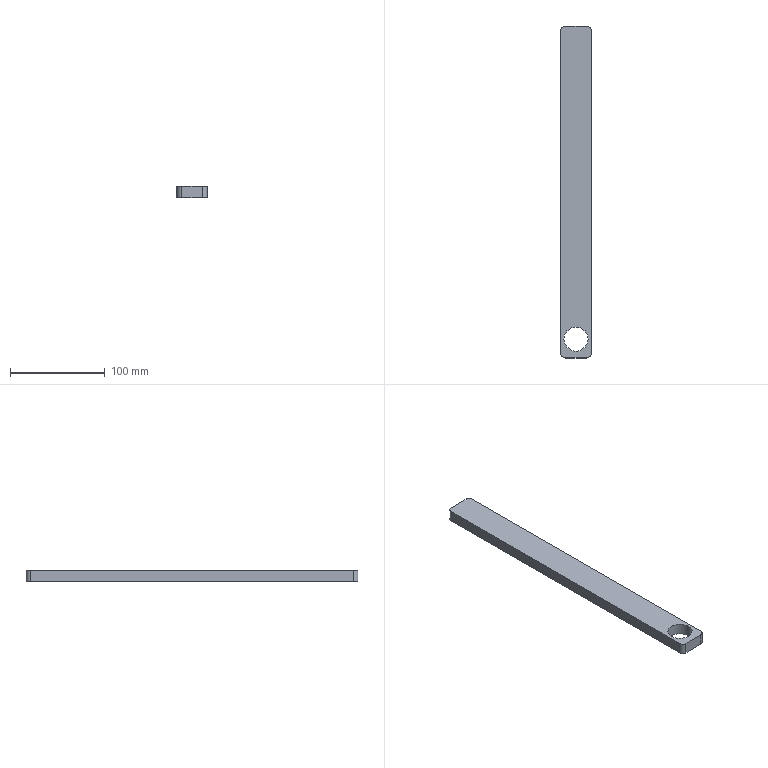Part | SolidWorks | features Extrusion 1 | 1 solid | 12 faces | box 32 x 350 x 12 mm | volume 128014 mm3 | cylinder 6 | plane 6 | commonest cylinder face diameters 10 x4 25.5 x2
STEP:
#1=CARTESIAN_POINT('',(3.25,20.,12.));
#2=VERTEX_POINT('',#1);
#3=CARTESIAN_POINT('',(28.75,20.,12.));
#4=VERTEX_POINT('',#3);
#5=CARTESIAN_POINT('',(16.,20.,12.));
#6=DIRECTION('',(0.,0.,1.));
#7=DIRECTION('',(1.,0.,0.));
#8=AXIS2_PLACEMENT_3D('',#5,#6,#7);
#9=CIRCLE('',#8,12.75);
#10=EDGE_CURVE('',#2,#4,#9,.T.);
#11=ORIENTED_EDGE('',*,*,#10,.T.);
#12=CARTESIAN_POINT('',(28.75,20.,0.));
#13=VERTEX_POINT('',#12);
#14=CARTESIAN_POINT('',(28.75,20.,12.));
#15=DIRECTION('',(0.,0.,-1.));
#16=VECTOR('',#15,1000.);
#17=LINE('',#14,#16);
#18=EDGE_CURVE('',#4,#13,#17,.T.);
#19=ORIENTED_EDGE('',*,*,#18,.T.);
#20=CARTESIAN_POINT('',(3.25,20.,0.));
#21=VERTEX_POINT('',#20);
#22=CARTESIAN_POINT('',(16.,20.,0.));
#23=DIRECTION('',(0.,0.,1.));
#24=DIRECTION('',(1.,0.,0.));
#25=AXIS2_PLACEMENT_3D('',#22,#23,#24);
#26=CIRCLE('',#25,12.75);
#27=EDGE_CURVE('',#21,#13,#26,.T.);
#28=ORIENTED_EDGE('',*,*,#27,.F.);
#29=CARTESIAN_POINT('',(3.25,20.,12.));
#30=DIRECTION('',(0.,0.,-1.));
#31=VECTOR('',#30,1000.);
#32=LINE('',#29,#31);
#33=EDGE_CURVE('',#2,#21,#32,.T.);
#34=ORIENTED_EDGE('',*,*,#33,.F.);
#35=EDGE_LOOP('',(#11,#19,#28,#34));
#36=FACE_OUTER_BOUND('',#35,.T.);
#37=CARTESIAN_POINT('',(16.,20.,12.));
#38=DIRECTION('',(0.,0.,-1.));
#39=DIRECTION('',(-1.,0.,0.));
#40=AXIS2_PLACEMENT_3D('',#37,#38,#39);
#41=CYLINDRICAL_SURFACE('',#40,12.75);
#42=ADVANCED_FACE('',(#36),#41,.F.);
#43=CARTESIAN_POINT('',(27.,0.,12.));
#44=VERTEX_POINT('',#43);
#45=CARTESIAN_POINT('',(32.,5.,12.));
#46=VERTEX_POINT('',#45);
#47=CARTESIAN_POINT('',(27.,5.,12.));
#48=DIRECTION('',(0.,0.,1.));
#49=DIRECTION('',(1.,0.,0.));
#50=AXIS2_PLACEMENT_3D('',#47,#48,#49);
#51=CIRCLE('',#50,5.);
#52=EDGE_CURVE('',#44,#46,#51,.T.);
#53=ORIENTED_EDGE('',*,*,#52,.T.);
#54=CARTESIAN_POINT('',(32.,345.,12.));
#55=VERTEX_POINT('',#54);
#56=CARTESIAN_POINT('',(32.,5.,12.));
#57=DIRECTION('',(0.,1.,0.));
#58=VECTOR('',#57,1000.);
#59=LINE('',#56,#58);
#60=EDGE_CURVE('',#46,#55,#59,.T.);
#61=ORIENTED_EDGE('',*,*,#60,.T.);
#62=CARTESIAN_POINT('',(27.,350.,12.));
#63=VERTEX_POINT('',#62);
#64=CARTESIAN_POINT('',(27.,345.,12.));
#65=DIRECTION('',(0.,0.,1.));
#66=DIRECTION('',(-1.,0.,0.));
#67=AXIS2_PLACEMENT_3D('',#64,#65,#66);
#68=CIRCLE('',#67,5.);
#69=EDGE_CURVE('',#55,#63,#68,.T.);
#70=ORIENTED_EDGE('',*,*,#69,.T.);
#71=CARTESIAN_POINT('',(5.,350.,12.));
#72=VERTEX_POINT('',#71);
#73=CARTESIAN_POINT('',(5.,350.,12.));
#74=DIRECTION('',(-1.,0.,0.));
#75=VECTOR('',#74,1000.);
#76=LINE('',#73,#75);
#77=EDGE_CURVE('',#63,#72,#76,.T.);
#78=ORIENTED_EDGE('',*,*,#77,.T.);
#79=CARTESIAN_POINT('',(0.,345.,12.));
#80=VERTEX_POINT('',#79);
#81=CARTESIAN_POINT('',(5.,345.,12.));
#82=DIRECTION('',(0.,0.,1.));
#83=DIRECTION('',(-1.,0.,0.));
#84=AXIS2_PLACEMENT_3D('',#81,#82,#83);
#85=CIRCLE('',#84,5.);
#86=EDGE_CURVE('',#72,#80,#85,.T.);
#87=ORIENTED_EDGE('',*,*,#86,.T.);
#88=CARTESIAN_POINT('',(0.,5.,12.));
#89=VERTEX_POINT('',#88);
#90=CARTESIAN_POINT('',(0.,5.,12.));
#91=DIRECTION('',(0.,-1.,0.));
#92=VECTOR('',#91,1000.);
#93=LINE('',#90,#92);
#94=EDGE_CURVE('',#80,#89,#93,.T.);
#95=ORIENTED_EDGE('',*,*,#94,.T.);
#96=CARTESIAN_POINT('',(5.,0.,12.));
#97=VERTEX_POINT('',#96);
#98=CARTESIAN_POINT('',(5.,5.,12.));
#99=DIRECTION('',(0.,0.,1.));
#100=DIRECTION('',(-1.,0.,0.));
#101=AXIS2_PLACEMENT_3D('',#98,#99,#100);
#102=CIRCLE('',#101,5.);
#103=EDGE_CURVE('',#89,#97,#102,.T.);
#104=ORIENTED_EDGE('',*,*,#103,.T.);
#105=CARTESIAN_POINT('',(5.,0.,12.));
#106=DIRECTION('',(1.,0.,0.));
#107=VECTOR('',#106,1000.);
#108=LINE('',#105,#107);
#109=EDGE_CURVE('',#97,#44,#108,.T.);
#110=ORIENTED_EDGE('',*,*,#109,.T.);
#111=EDGE_LOOP('',(#53,#61,#70,#78,#87,#95,#104,#110));
#112=FACE_OUTER_BOUND('',#111,.T.);
#113=ORIENTED_EDGE('',*,*,#10,.F.);
#114=CARTESIAN_POINT('',(16.,20.,12.));
#115=DIRECTION('',(0.,0.,1.));
#116=DIRECTION('',(1.,0.,0.));
#117=AXIS2_PLACEMENT_3D('',#114,#115,#116);
#118=CIRCLE('',#117,12.75);
#119=EDGE_CURVE('',#4,#2,#118,.T.);
#120=ORIENTED_EDGE('',*,*,#119,.F.);
#121=EDGE_LOOP('',(#113,#120));
#122=FACE_BOUND('',#121,.T.);
#123=CARTESIAN_POINT('',(27.,5.,12.));
#124=DIRECTION('',(0.,0.,1.));
#125=DIRECTION('',(1.,0.,0.));
#126=AXIS2_PLACEMENT_3D('',#123,#124,#125);
#127=PLANE('',#126);
#128=ADVANCED_FACE('',(#112,#122),#127,.T.);
#129=CARTESIAN_POINT('',(27.,0.,0.));
#130=VERTEX_POINT('',#129);
#131=CARTESIAN_POINT('',(32.,5.,0.));
#132=VERTEX_POINT('',#131);
#133=CARTESIAN_POINT('',(27.,5.,0.));
#134=DIRECTION('',(0.,0.,1.));
#135=DIRECTION('',(1.,0.,0.));
#136=AXIS2_PLACEMENT_3D('',#133,#134,#135);
#137=CIRCLE('',#136,5.);
#138=EDGE_CURVE('',#130,#132,#137,.T.);
#139=ORIENTED_EDGE('',*,*,#138,.F.);
#140=CARTESIAN_POINT('',(5.,0.,0.));
#141=VERTEX_POINT('',#140);
#142=CARTESIAN_POINT('',(5.,0.,0.));
#143=DIRECTION('',(1.,0.,0.));
#144=VECTOR('',#143,1000.);
#145=LINE('',#142,#144);
#146=EDGE_CURVE('',#141,#130,#145,.T.);
#147=ORIENTED_EDGE('',*,*,#146,.F.);
#148=CARTESIAN_POINT('',(0.,5.,0.));
#149=VERTEX_POINT('',#148);
#150=CARTESIAN_POINT('',(5.,5.,0.));
#151=DIRECTION('',(0.,0.,1.));
#152=DIRECTION('',(-1.,0.,0.));
#153=AXIS2_PLACEMENT_3D('',#150,#151,#152);
#154=CIRCLE('',#153,5.);
#155=EDGE_CURVE('',#149,#141,#154,.T.);
#156=ORIENTED_EDGE('',*,*,#155,.F.);
#157=CARTESIAN_POINT('',(0.,345.,0.));
#158=VERTEX_POINT('',#157);
#159=CARTESIAN_POINT('',(0.,5.,0.));
#160=DIRECTION('',(0.,-1.,0.));
#161=VECTOR('',#160,1000.);
#162=LINE('',#159,#161);
#163=EDGE_CURVE('',#158,#149,#162,.T.);
#164=ORIENTED_EDGE('',*,*,#163,.F.);
#165=CARTESIAN_POINT('',(5.,350.,0.));
#166=VERTEX_POINT('',#165);
#167=CARTESIAN_POINT('',(5.,345.,0.));
#168=DIRECTION('',(0.,0.,1.));
#169=DIRECTION('',(-1.,0.,0.));
#170=AXIS2_PLACEMENT_3D('',#167,#168,#169);
#171=CIRCLE('',#170,5.);
#172=EDGE_CURVE('',#166,#158,#171,.T.);
#173=ORIENTED_EDGE('',*,*,#172,.F.);
#174=CARTESIAN_POINT('',(27.,350.,0.));
#175=VERTEX_POINT('',#174);
#176=CARTESIAN_POINT('',(5.,350.,0.));
#177=DIRECTION('',(-1.,0.,0.));
#178=VECTOR('',#177,1000.);
#179=LINE('',#176,#178);
#180=EDGE_CURVE('',#175,#166,#179,.T.);
#181=ORIENTED_EDGE('',*,*,#180,.F.);
#182=CARTESIAN_POINT('',(32.,345.,0.));
#183=VERTEX_POINT('',#182);
#184=CARTESIAN_POINT('',(27.,345.,0.));
#185=DIRECTION('',(0.,0.,1.));
#186=DIRECTION('',(-1.,0.,0.));
#187=AXIS2_PLACEMENT_3D('',#184,#185,#186);
#188=CIRCLE('',#187,5.);
#189=EDGE_CURVE('',#183,#175,#188,.T.);
#190=ORIENTED_EDGE('',*,*,#189,.F.);
#191=CARTESIAN_POINT('',(32.,5.,0.));
#192=DIRECTION('',(0.,1.,0.));
#193=VECTOR('',#192,1000.);
#194=LINE('',#191,#193);
#195=EDGE_CURVE('',#132,#183,#194,.T.);
#196=ORIENTED_EDGE('',*,*,#195,.F.);
#197=EDGE_LOOP('',(#139,#147,#156,#164,#173,#181,#190,#196));
#198=FACE_OUTER_BOUND('',#197,.T.);
#199=ORIENTED_EDGE('',*,*,#27,.T.);
#200=CARTESIAN_POINT('',(16.,20.,0.));
#201=DIRECTION('',(0.,0.,1.));
#202=DIRECTION('',(1.,0.,0.));
#203=AXIS2_PLACEMENT_3D('',#200,#201,#202);
#204=CIRCLE('',#203,12.75);
#205=EDGE_CURVE('',#13,#21,#204,.T.);
#206=ORIENTED_EDGE('',*,*,#205,.T.);
#207=EDGE_LOOP('',(#199,#206));
#208=FACE_BOUND('',#207,.T.);
#209=CARTESIAN_POINT('',(27.,5.,0.));
#210=DIRECTION('',(0.,0.,1.));
#211=DIRECTION('',(1.,0.,0.));
#212=AXIS2_PLACEMENT_3D('',#209,#210,#211);
#213=PLANE('',#212);
#214=ADVANCED_FACE('',(#198,#208),#213,.F.);
#215=ORIENTED_EDGE('',*,*,#138,.T.);
#216=CARTESIAN_POINT('',(32.,5.,12.));
#217=DIRECTION('',(0.,0.,-1.));
#218=VECTOR('',#217,1000.);
#219=LINE('',#216,#218);
#220=EDGE_CURVE('',#46,#132,#219,.T.);
#221=ORIENTED_EDGE('',*,*,#220,.F.);
#222=ORIENTED_EDGE('',*,*,#52,.F.);
#223=CARTESIAN_POINT('',(27.,0.,12.));
#224=DIRECTION('',(0.,0.,-1.));
#225=VECTOR('',#224,1000.);
#226=LINE('',#223,#225);
#227=EDGE_CURVE('',#44,#130,#226,.T.);
#228=ORIENTED_EDGE('',*,*,#227,.T.);
#229=EDGE_LOOP('',(#215,#221,#222,#228));
#230=FACE_OUTER_BOUND('',#229,.T.);
#231=CARTESIAN_POINT('',(27.,5.,12.));
#232=DIRECTION('',(0.,0.,-1.));
#233=DIRECTION('',(-1.,0.,0.));
#234=AXIS2_PLACEMENT_3D('',#231,#232,#233);
#235=CYLINDRICAL_SURFACE('',#234,5.);
#236=ADVANCED_FACE('',(#230),#235,.T.);
#237=ORIENTED_EDGE('',*,*,#195,.T.);
#238=CARTESIAN_POINT('',(32.,345.,12.));
#239=DIRECTION('',(0.,0.,-1.));
#240=VECTOR('',#239,1000.);
#241=LINE('',#238,#240);
#242=EDGE_CURVE('',#55,#183,#241,.T.);
#243=ORIENTED_EDGE('',*,*,#242,.F.);
#244=ORIENTED_EDGE('',*,*,#60,.F.);
#245=ORIENTED_EDGE('',*,*,#220,.T.);
#246=EDGE_LOOP('',(#237,#243,#244,#245));
#247=FACE_OUTER_BOUND('',#246,.T.);
#248=CARTESIAN_POINT('',(32.,5.,12.));
#249=DIRECTION('',(-1.,0.,0.));
#250=DIRECTION('',(0.,0.,1.));
#251=AXIS2_PLACEMENT_3D('',#248,#249,#250);
#252=PLANE('',#251);
#253=ADVANCED_FACE('',(#247),#252,.F.);
#254=ORIENTED_EDGE('',*,*,#189,.T.);
#255=CARTESIAN_POINT('',(27.,350.,12.));
#256=DIRECTION('',(0.,0.,-1.));
#257=VECTOR('',#256,1000.);
#258=LINE('',#255,#257);
#259=EDGE_CURVE('',#63,#175,#258,.T.);
#260=ORIENTED_EDGE('',*,*,#259,.F.);
#261=ORIENTED_EDGE('',*,*,#69,.F.);
#262=ORIENTED_EDGE('',*,*,#242,.T.);
#263=EDGE_LOOP('',(#254,#260,#261,#262));
#264=FACE_OUTER_BOUND('',#263,.T.);
#265=CARTESIAN_POINT('',(27.,345.,12.));
#266=DIRECTION('',(0.,0.,-1.));
#267=DIRECTION('',(-1.,0.,0.));
#268=AXIS2_PLACEMENT_3D('',#265,#266,#267);
#269=CYLINDRICAL_SURFACE('',#268,5.);
#270=ADVANCED_FACE('',(#264),#269,.T.);
#271=ORIENTED_EDGE('',*,*,#180,.T.);
#272=CARTESIAN_POINT('',(5.,350.,12.));
#273=DIRECTION('',(0.,0.,-1.));
#274=VECTOR('',#273,1000.);
#275=LINE('',#272,#274);
#276=EDGE_CURVE('',#72,#166,#275,.T.);
#277=ORIENTED_EDGE('',*,*,#276,.F.);
#278=ORIENTED_EDGE('',*,*,#77,.F.);
#279=ORIENTED_EDGE('',*,*,#259,.T.);
#280=EDGE_LOOP('',(#271,#277,#278,#279));
#281=FACE_OUTER_BOUND('',#280,.T.);
#282=CARTESIAN_POINT('',(5.,350.,12.));
#283=DIRECTION('',(0.,-1.,0.));
#284=DIRECTION('',(0.,0.,-1.));
#285=AXIS2_PLACEMENT_3D('',#282,#283,#284);
#286=PLANE('',#285);
#287=ADVANCED_FACE('',(#281),#286,.F.);
#288=ORIENTED_EDGE('',*,*,#172,.T.);
#289=CARTESIAN_POINT('',(0.,345.,12.));
#290=DIRECTION('',(0.,0.,-1.));
#291=VECTOR('',#290,1000.);
#292=LINE('',#289,#291);
#293=EDGE_CURVE('',#80,#158,#292,.T.);
#294=ORIENTED_EDGE('',*,*,#293,.F.);
#295=ORIENTED_EDGE('',*,*,#86,.F.);
#296=ORIENTED_EDGE('',*,*,#276,.T.);
#297=EDGE_LOOP('',(#288,#294,#295,#296));
#298=FACE_OUTER_BOUND('',#297,.T.);
#299=CARTESIAN_POINT('',(5.,345.,12.));
#300=DIRECTION('',(0.,0.,-1.));
#301=DIRECTION('',(-1.,0.,0.));
#302=AXIS2_PLACEMENT_3D('',#299,#300,#301);
#303=CYLINDRICAL_SURFACE('',#302,5.);
#304=ADVANCED_FACE('',(#298),#303,.T.);
#305=ORIENTED_EDGE('',*,*,#163,.T.);
#306=CARTESIAN_POINT('',(0.,5.,12.));
#307=DIRECTION('',(0.,0.,-1.));
#308=VECTOR('',#307,1000.);
#309=LINE('',#306,#308);
#310=EDGE_CURVE('',#89,#149,#309,.T.);
#311=ORIENTED_EDGE('',*,*,#310,.F.);
#312=ORIENTED_EDGE('',*,*,#94,.F.);
#313=ORIENTED_EDGE('',*,*,#293,.T.);
#314=EDGE_LOOP('',(#305,#311,#312,#313));
#315=FACE_OUTER_BOUND('',#314,.T.);
#316=CARTESIAN_POINT('',(0.,5.,12.));
#317=DIRECTION('',(1.,0.,0.));
#318=DIRECTION('',(0.,0.,-1.));
#319=AXIS2_PLACEMENT_3D('',#316,#317,#318);
#320=PLANE('',#319);
#321=ADVANCED_FACE('',(#315),#320,.F.);
#322=ORIENTED_EDGE('',*,*,#155,.T.);
#323=CARTESIAN_POINT('',(5.,0.,12.));
#324=DIRECTION('',(0.,0.,-1.));
#325=VECTOR('',#324,1000.);
#326=LINE('',#323,#325);
#327=EDGE_CURVE('',#97,#141,#326,.T.);
#328=ORIENTED_EDGE('',*,*,#327,.F.);
#329=ORIENTED_EDGE('',*,*,#103,.F.);
#330=ORIENTED_EDGE('',*,*,#310,.T.);
#331=EDGE_LOOP('',(#322,#328,#329,#330));
#332=FACE_OUTER_BOUND('',#331,.T.);
#333=CARTESIAN_POINT('',(5.,5.,12.));
#334=DIRECTION('',(0.,0.,-1.));
#335=DIRECTION('',(-1.,0.,0.));
#336=AXIS2_PLACEMENT_3D('',#333,#334,#335);
#337=CYLINDRICAL_SURFACE('',#336,5.);
#338=ADVANCED_FACE('',(#332),#337,.T.);
#339=ORIENTED_EDGE('',*,*,#146,.T.);
#340=ORIENTED_EDGE('',*,*,#227,.F.);
#341=ORIENTED_EDGE('',*,*,#109,.F.);
#342=ORIENTED_EDGE('',*,*,#327,.T.);
#343=EDGE_LOOP('',(#339,#340,#341,#342));
#344=FACE_OUTER_BOUND('',#343,.T.);
#345=CARTESIAN_POINT('',(5.,0.,12.));
#346=DIRECTION('',(0.,1.,0.));
#347=DIRECTION('',(0.,0.,1.));
#348=AXIS2_PLACEMENT_3D('',#345,#346,#347);
#349=PLANE('',#348);
#350=ADVANCED_FACE('',(#344),#349,.F.);
#351=ORIENTED_EDGE('',*,*,#18,.F.);
#352=ORIENTED_EDGE('',*,*,#119,.T.);
#353=ORIENTED_EDGE('',*,*,#33,.T.);
#354=ORIENTED_EDGE('',*,*,#205,.F.);
#355=EDGE_LOOP('',(#351,#352,#353,#354));
#356=FACE_OUTER_BOUND('',#355,.T.);
#357=CARTESIAN_POINT('',(16.,20.,12.));
#358=DIRECTION('',(0.,0.,-1.));
#359=DIRECTION('',(-1.,0.,0.));
#360=AXIS2_PLACEMENT_3D('',#357,#358,#359);
#361=CYLINDRICAL_SURFACE('',#360,12.75);
#362=ADVANCED_FACE('',(#356),#361,.F.);
#363=CLOSED_SHELL('',(#42,#128,#214,#236,#253,#270,#287,#304,#321,#338,#350,#362));
#364=MANIFOLD_SOLID_BREP('',#363);
#365=CARTESIAN_POINT('',(0.,0.,0.));
#366=DIRECTION('',(0.,0.,1.));
#367=DIRECTION('',(1.,0.,0.));
#368=AXIS2_PLACEMENT_3D('',#365,#366,#367);
#369=(LENGTH_UNIT()NAMED_UNIT(*)SI_UNIT(.MILLI.,.METRE.));
#370=UNCERTAINTY_MEASURE_WITH_UNIT(LENGTH_MEASURE(0.00001),#369,'','');
#371=(NAMED_UNIT(*)PLANE_ANGLE_UNIT()SI_UNIT($,.RADIAN.));
#372=(NAMED_UNIT(*)SI_UNIT($,.STERADIAN.)SOLID_ANGLE_UNIT());
#373=(GEOMETRIC_REPRESENTATION_CONTEXT(3)GLOBAL_UNCERTAINTY_ASSIGNED_CONTEXT((#370))GLOBAL_UNIT_ASSIGNED_CONTEXT((#369,#371,#372))REPRESENTATION_CONTEXT('',''));
#374=ADVANCED_BREP_SHAPE_REPRESENTATION('',(#364,#368),#373);